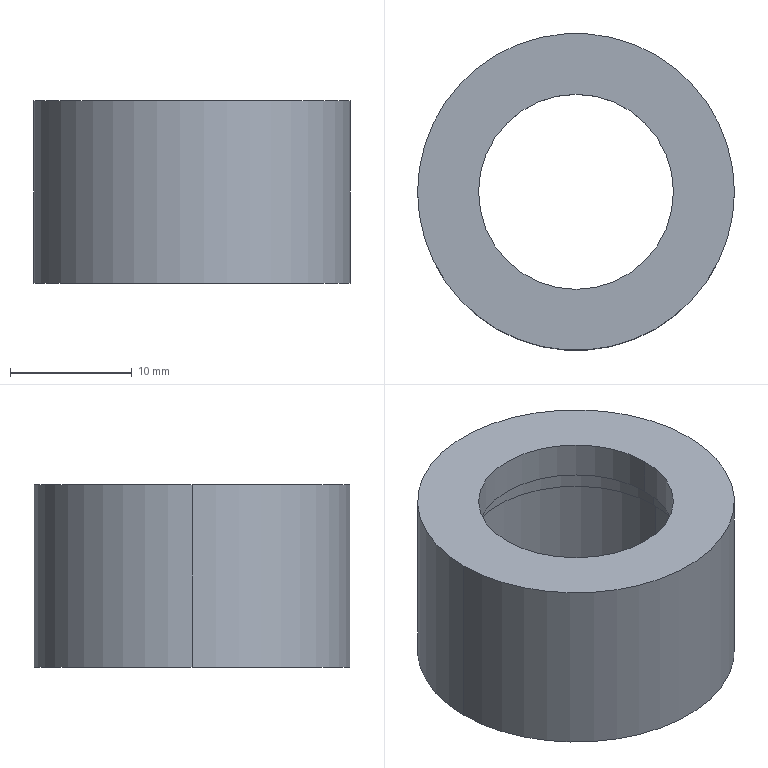Part | SolidWorks | features Revolution 1 | 1 solid | 13 faces | box 26 x 26 x 15 mm | volume 4163 mm3 | cylinder 8 | plane 3 | cone 2 | commonest cylinder face diameters 16 x2 18 x2 18.5 x2 26 x2
STEP:
#1=CARTESIAN_POINT('',(9.,0.,10.15));
#2=VERTEX_POINT('',#1);
#3=CARTESIAN_POINT('',(-9.,0.,10.15));
#4=VERTEX_POINT('',#3);
#5=CARTESIAN_POINT('',(0.,0.,10.15));
#6=DIRECTION('',(0.,0.,-1.));
#7=DIRECTION('',(-1.,0.,0.));
#8=AXIS2_PLACEMENT_3D('',#5,#6,#7);
#9=CIRCLE('',#8,9.);
#10=EDGE_CURVE('',#2,#4,#9,.T.);
#11=ORIENTED_EDGE('',*,*,#10,.F.);
#12=CARTESIAN_POINT('',(9.25,0.,10.));
#13=VERTEX_POINT('',#12);
#14=CARTESIAN_POINT('',(9.,0.,10.15));
#15=DIRECTION('',(0.8572,0.,-0.515));
#16=VECTOR('',#15,1000.);
#17=LINE('',#14,#16);
#18=EDGE_CURVE('',#2,#13,#17,.T.);
#19=ORIENTED_EDGE('',*,*,#18,.T.);
#20=CARTESIAN_POINT('',(-9.25,0.,10.));
#21=VERTEX_POINT('',#20);
#22=CARTESIAN_POINT('',(0.,0.,10.));
#23=DIRECTION('',(0.,0.,-1.));
#24=DIRECTION('',(-1.,0.,0.));
#25=AXIS2_PLACEMENT_3D('',#22,#23,#24);
#26=CIRCLE('',#25,9.25);
#27=EDGE_CURVE('',#13,#21,#26,.T.);
#28=ORIENTED_EDGE('',*,*,#27,.T.);
#29=CARTESIAN_POINT('',(-9.,0.,10.15));
#30=DIRECTION('',(-0.8572,0.,-0.515));
#31=VECTOR('',#30,1000.);
#32=LINE('',#29,#31);
#33=EDGE_CURVE('',#4,#21,#32,.T.);
#34=ORIENTED_EDGE('',*,*,#33,.F.);
#35=EDGE_LOOP('',(#11,#19,#28,#34));
#36=FACE_OUTER_BOUND('',#35,.T.);
#37=CARTESIAN_POINT('',(0.,0.,10.15));
#38=DIRECTION('',(0.,0.,-1.));
#39=DIRECTION('',(-1.,0.,0.));
#40=AXIS2_PLACEMENT_3D('',#37,#38,#39);
#41=CONICAL_SURFACE('',#40,9.,1.03);
#42=ADVANCED_FACE('',(#36),#41,.F.);
#43=CARTESIAN_POINT('',(9.,0.,12.));
#44=VERTEX_POINT('',#43);
#45=CARTESIAN_POINT('',(-9.,0.,12.));
#46=VERTEX_POINT('',#45);
#47=CARTESIAN_POINT('',(0.,0.,12.));
#48=DIRECTION('',(0.,0.,-1.));
#49=DIRECTION('',(-1.,0.,0.));
#50=AXIS2_PLACEMENT_3D('',#47,#48,#49);
#51=CIRCLE('',#50,9.);
#52=EDGE_CURVE('',#44,#46,#51,.T.);
#53=ORIENTED_EDGE('',*,*,#52,.F.);
#54=CARTESIAN_POINT('',(9.,0.,15.));
#55=DIRECTION('',(0.,0.,-1.));
#56=VECTOR('',#55,1000.);
#57=LINE('',#54,#56);
#58=EDGE_CURVE('',#44,#2,#57,.T.);
#59=ORIENTED_EDGE('',*,*,#58,.T.);
#60=ORIENTED_EDGE('',*,*,#10,.T.);
#61=CARTESIAN_POINT('',(-9.,0.,15.));
#62=DIRECTION('',(0.,0.,-1.));
#63=VECTOR('',#62,1000.);
#64=LINE('',#61,#63);
#65=EDGE_CURVE('',#46,#4,#64,.T.);
#66=ORIENTED_EDGE('',*,*,#65,.F.);
#67=EDGE_LOOP('',(#53,#59,#60,#66));
#68=FACE_OUTER_BOUND('',#67,.T.);
#69=CARTESIAN_POINT('',(0.,0.,15.));
#70=DIRECTION('',(0.,0.,-1.));
#71=DIRECTION('',(-1.,0.,0.));
#72=AXIS2_PLACEMENT_3D('',#69,#70,#71);
#73=CYLINDRICAL_SURFACE('',#72,9.);
#74=ADVANCED_FACE('',(#68),#73,.F.);
#75=CARTESIAN_POINT('',(8.,0.,15.));
#76=VERTEX_POINT('',#75);
#77=CARTESIAN_POINT('',(-8.,0.,15.));
#78=VERTEX_POINT('',#77);
#79=CARTESIAN_POINT('',(0.,0.,15.));
#80=DIRECTION('',(0.,0.,-1.));
#81=DIRECTION('',(-1.,0.,0.));
#82=AXIS2_PLACEMENT_3D('',#79,#80,#81);
#83=CIRCLE('',#82,8.);
#84=EDGE_CURVE('',#76,#78,#83,.T.);
#85=ORIENTED_EDGE('',*,*,#84,.F.);
#86=CARTESIAN_POINT('',(8.,0.,12.));
#87=VERTEX_POINT('',#86);
#88=CARTESIAN_POINT('',(8.,0.,15.));
#89=DIRECTION('',(0.,0.,-1.));
#90=VECTOR('',#89,1000.);
#91=LINE('',#88,#90);
#92=EDGE_CURVE('',#76,#87,#91,.T.);
#93=ORIENTED_EDGE('',*,*,#92,.T.);
#94=CARTESIAN_POINT('',(-8.,0.,12.));
#95=VERTEX_POINT('',#94);
#96=CARTESIAN_POINT('',(0.,0.,12.));
#97=DIRECTION('',(0.,0.,-1.));
#98=DIRECTION('',(-1.,0.,0.));
#99=AXIS2_PLACEMENT_3D('',#96,#97,#98);
#100=CIRCLE('',#99,8.);
#101=EDGE_CURVE('',#87,#95,#100,.T.);
#102=ORIENTED_EDGE('',*,*,#101,.T.);
#103=CARTESIAN_POINT('',(-8.,0.,15.));
#104=DIRECTION('',(0.,0.,-1.));
#105=VECTOR('',#104,1000.);
#106=LINE('',#103,#105);
#107=EDGE_CURVE('',#78,#95,#106,.T.);
#108=ORIENTED_EDGE('',*,*,#107,.F.);
#109=EDGE_LOOP('',(#85,#93,#102,#108));
#110=FACE_OUTER_BOUND('',#109,.T.);
#111=CARTESIAN_POINT('',(0.,0.,15.));
#112=DIRECTION('',(0.,0.,-1.));
#113=DIRECTION('',(-1.,0.,0.));
#114=AXIS2_PLACEMENT_3D('',#111,#112,#113);
#115=CYLINDRICAL_SURFACE('',#114,8.);
#116=ADVANCED_FACE('',(#110),#115,.F.);
#117=CARTESIAN_POINT('',(-13.,0.,15.));
#118=VERTEX_POINT('',#117);
#119=CARTESIAN_POINT('',(13.,0.,15.));
#120=VERTEX_POINT('',#119);
#121=CARTESIAN_POINT('',(0.,0.,15.));
#122=DIRECTION('',(0.,0.,-1.));
#123=DIRECTION('',(-1.,0.,0.));
#124=AXIS2_PLACEMENT_3D('',#121,#122,#123);
#125=CIRCLE('',#124,13.);
#126=EDGE_CURVE('',#118,#120,#125,.T.);
#127=ORIENTED_EDGE('',*,*,#126,.T.);
#128=CARTESIAN_POINT('',(13.,0.,0.));
#129=VERTEX_POINT('',#128);
#130=CARTESIAN_POINT('',(13.,0.,15.));
#131=DIRECTION('',(0.,0.,-1.));
#132=VECTOR('',#131,1000.);
#133=LINE('',#130,#132);
#134=EDGE_CURVE('',#120,#129,#133,.T.);
#135=ORIENTED_EDGE('',*,*,#134,.T.);
#136=CARTESIAN_POINT('',(-13.,0.,0.));
#137=VERTEX_POINT('',#136);
#138=CARTESIAN_POINT('',(0.,0.,0.));
#139=DIRECTION('',(0.,0.,-1.));
#140=DIRECTION('',(-1.,0.,0.));
#141=AXIS2_PLACEMENT_3D('',#138,#139,#140);
#142=CIRCLE('',#141,13.);
#143=EDGE_CURVE('',#137,#129,#142,.T.);
#144=ORIENTED_EDGE('',*,*,#143,.F.);
#145=CARTESIAN_POINT('',(-13.,0.,15.));
#146=DIRECTION('',(0.,0.,-1.));
#147=VECTOR('',#146,1000.);
#148=LINE('',#145,#147);
#149=EDGE_CURVE('',#118,#137,#148,.T.);
#150=ORIENTED_EDGE('',*,*,#149,.F.);
#151=EDGE_LOOP('',(#127,#135,#144,#150));
#152=FACE_OUTER_BOUND('',#151,.T.);
#153=CARTESIAN_POINT('',(0.,0.,15.));
#154=DIRECTION('',(0.,0.,-1.));
#155=DIRECTION('',(-1.,0.,0.));
#156=AXIS2_PLACEMENT_3D('',#153,#154,#155);
#157=CYLINDRICAL_SURFACE('',#156,13.);
#158=ADVANCED_FACE('',(#152),#157,.T.);
#159=ORIENTED_EDGE('',*,*,#27,.F.);
#160=CARTESIAN_POINT('',(9.25,0.,0.));
#161=VERTEX_POINT('',#160);
#162=CARTESIAN_POINT('',(9.25,0.,15.));
#163=DIRECTION('',(0.,0.,-1.));
#164=VECTOR('',#163,1000.);
#165=LINE('',#162,#164);
#166=EDGE_CURVE('',#13,#161,#165,.T.);
#167=ORIENTED_EDGE('',*,*,#166,.T.);
#168=CARTESIAN_POINT('',(-9.25,0.,0.));
#169=VERTEX_POINT('',#168);
#170=CARTESIAN_POINT('',(0.,0.,0.));
#171=DIRECTION('',(0.,0.,-1.));
#172=DIRECTION('',(-1.,0.,0.));
#173=AXIS2_PLACEMENT_3D('',#170,#171,#172);
#174=CIRCLE('',#173,9.25);
#175=EDGE_CURVE('',#161,#169,#174,.T.);
#176=ORIENTED_EDGE('',*,*,#175,.T.);
#177=CARTESIAN_POINT('',(-9.25,0.,15.));
#178=DIRECTION('',(0.,0.,-1.));
#179=VECTOR('',#178,1000.);
#180=LINE('',#177,#179);
#181=EDGE_CURVE('',#21,#169,#180,.T.);
#182=ORIENTED_EDGE('',*,*,#181,.F.);
#183=EDGE_LOOP('',(#159,#167,#176,#182));
#184=FACE_OUTER_BOUND('',#183,.T.);
#185=CARTESIAN_POINT('',(0.,0.,15.));
#186=DIRECTION('',(0.,0.,-1.));
#187=DIRECTION('',(-1.,0.,0.));
#188=AXIS2_PLACEMENT_3D('',#185,#186,#187);
#189=CYLINDRICAL_SURFACE('',#188,9.25);
#190=ADVANCED_FACE('',(#184),#189,.F.);
#191=ORIENTED_EDGE('',*,*,#166,.F.);
#192=CARTESIAN_POINT('',(0.,0.,10.));
#193=DIRECTION('',(0.,0.,-1.));
#194=DIRECTION('',(-1.,0.,0.));
#195=AXIS2_PLACEMENT_3D('',#192,#193,#194);
#196=CIRCLE('',#195,9.25);
#197=EDGE_CURVE('',#21,#13,#196,.T.);
#198=ORIENTED_EDGE('',*,*,#197,.F.);
#199=ORIENTED_EDGE('',*,*,#181,.T.);
#200=CARTESIAN_POINT('',(0.,0.,0.));
#201=DIRECTION('',(0.,0.,-1.));
#202=DIRECTION('',(-1.,0.,0.));
#203=AXIS2_PLACEMENT_3D('',#200,#201,#202);
#204=CIRCLE('',#203,9.25);
#205=EDGE_CURVE('',#169,#161,#204,.T.);
#206=ORIENTED_EDGE('',*,*,#205,.T.);
#207=EDGE_LOOP('',(#191,#198,#199,#206));
#208=FACE_OUTER_BOUND('',#207,.T.);
#209=CARTESIAN_POINT('',(0.,0.,15.));
#210=DIRECTION('',(0.,0.,-1.));
#211=DIRECTION('',(-1.,0.,0.));
#212=AXIS2_PLACEMENT_3D('',#209,#210,#211);
#213=CYLINDRICAL_SURFACE('',#212,9.25);
#214=ADVANCED_FACE('',(#208),#213,.F.);
#215=ORIENTED_EDGE('',*,*,#143,.T.);
#216=CARTESIAN_POINT('',(0.,0.,0.));
#217=DIRECTION('',(0.,0.,-1.));
#218=DIRECTION('',(-1.,0.,0.));
#219=AXIS2_PLACEMENT_3D('',#216,#217,#218);
#220=CIRCLE('',#219,13.);
#221=EDGE_CURVE('',#129,#137,#220,.T.);
#222=ORIENTED_EDGE('',*,*,#221,.T.);
#223=EDGE_LOOP('',(#215,#222));
#224=FACE_OUTER_BOUND('',#223,.T.);
#225=ORIENTED_EDGE('',*,*,#205,.F.);
#226=ORIENTED_EDGE('',*,*,#175,.F.);
#227=EDGE_LOOP('',(#225,#226));
#228=FACE_BOUND('',#227,.T.);
#229=CARTESIAN_POINT('',(9.25,0.,0.));
#230=DIRECTION('',(0.,0.,-1.));
#231=DIRECTION('',(-1.,0.,0.));
#232=AXIS2_PLACEMENT_3D('',#229,#230,#231);
#233=PLANE('',#232);
#234=ADVANCED_FACE('',(#224,#228),#233,.T.);
#235=ORIENTED_EDGE('',*,*,#134,.F.);
#236=CARTESIAN_POINT('',(0.,0.,15.));
#237=DIRECTION('',(0.,0.,-1.));
#238=DIRECTION('',(-1.,0.,0.));
#239=AXIS2_PLACEMENT_3D('',#236,#237,#238);
#240=CIRCLE('',#239,13.);
#241=EDGE_CURVE('',#120,#118,#240,.T.);
#242=ORIENTED_EDGE('',*,*,#241,.T.);
#243=ORIENTED_EDGE('',*,*,#149,.T.);
#244=ORIENTED_EDGE('',*,*,#221,.F.);
#245=EDGE_LOOP('',(#235,#242,#243,#244));
#246=FACE_OUTER_BOUND('',#245,.T.);
#247=CARTESIAN_POINT('',(0.,0.,15.));
#248=DIRECTION('',(0.,0.,-1.));
#249=DIRECTION('',(-1.,0.,0.));
#250=AXIS2_PLACEMENT_3D('',#247,#248,#249);
#251=CYLINDRICAL_SURFACE('',#250,13.);
#252=ADVANCED_FACE('',(#246),#251,.T.);
#253=CARTESIAN_POINT('',(0.,0.,15.));
#254=DIRECTION('',(0.,0.,-1.));
#255=DIRECTION('',(-1.,0.,0.));
#256=AXIS2_PLACEMENT_3D('',#253,#254,#255);
#257=CIRCLE('',#256,8.);
#258=EDGE_CURVE('',#78,#76,#257,.T.);
#259=ORIENTED_EDGE('',*,*,#258,.T.);
#260=ORIENTED_EDGE('',*,*,#84,.T.);
#261=EDGE_LOOP('',(#259,#260));
#262=FACE_BOUND('',#261,.T.);
#263=ORIENTED_EDGE('',*,*,#126,.F.);
#264=ORIENTED_EDGE('',*,*,#241,.F.);
#265=EDGE_LOOP('',(#263,#264));
#266=FACE_OUTER_BOUND('',#265,.T.);
#267=CARTESIAN_POINT('',(13.,0.,15.));
#268=DIRECTION('',(0.,0.,1.));
#269=DIRECTION('',(1.,0.,0.));
#270=AXIS2_PLACEMENT_3D('',#267,#268,#269);
#271=PLANE('',#270);
#272=ADVANCED_FACE('',(#262,#266),#271,.T.);
#273=ORIENTED_EDGE('',*,*,#92,.F.);
#274=ORIENTED_EDGE('',*,*,#258,.F.);
#275=ORIENTED_EDGE('',*,*,#107,.T.);
#276=CARTESIAN_POINT('',(0.,0.,12.));
#277=DIRECTION('',(0.,0.,-1.));
#278=DIRECTION('',(-1.,0.,0.));
#279=AXIS2_PLACEMENT_3D('',#276,#277,#278);
#280=CIRCLE('',#279,8.);
#281=EDGE_CURVE('',#95,#87,#280,.T.);
#282=ORIENTED_EDGE('',*,*,#281,.T.);
#283=EDGE_LOOP('',(#273,#274,#275,#282));
#284=FACE_OUTER_BOUND('',#283,.T.);
#285=CARTESIAN_POINT('',(0.,0.,15.));
#286=DIRECTION('',(0.,0.,-1.));
#287=DIRECTION('',(-1.,0.,0.));
#288=AXIS2_PLACEMENT_3D('',#285,#286,#287);
#289=CYLINDRICAL_SURFACE('',#288,8.);
#290=ADVANCED_FACE('',(#284),#289,.F.);
#291=CARTESIAN_POINT('',(0.,0.,12.));
#292=DIRECTION('',(0.,0.,-1.));
#293=DIRECTION('',(-1.,0.,0.));
#294=AXIS2_PLACEMENT_3D('',#291,#292,#293);
#295=CIRCLE('',#294,9.);
#296=EDGE_CURVE('',#46,#44,#295,.T.);
#297=ORIENTED_EDGE('',*,*,#296,.T.);
#298=ORIENTED_EDGE('',*,*,#52,.T.);
#299=EDGE_LOOP('',(#297,#298));
#300=FACE_OUTER_BOUND('',#299,.T.);
#301=ORIENTED_EDGE('',*,*,#281,.F.);
#302=ORIENTED_EDGE('',*,*,#101,.F.);
#303=EDGE_LOOP('',(#301,#302));
#304=FACE_BOUND('',#303,.T.);
#305=CARTESIAN_POINT('',(8.,0.,12.));
#306=DIRECTION('',(0.,0.,-1.));
#307=DIRECTION('',(-1.,0.,0.));
#308=AXIS2_PLACEMENT_3D('',#305,#306,#307);
#309=PLANE('',#308);
#310=ADVANCED_FACE('',(#300,#304),#309,.T.);
#311=ORIENTED_EDGE('',*,*,#58,.F.);
#312=ORIENTED_EDGE('',*,*,#296,.F.);
#313=ORIENTED_EDGE('',*,*,#65,.T.);
#314=CARTESIAN_POINT('',(0.,0.,10.15));
#315=DIRECTION('',(0.,0.,-1.));
#316=DIRECTION('',(-1.,0.,0.));
#317=AXIS2_PLACEMENT_3D('',#314,#315,#316);
#318=CIRCLE('',#317,9.);
#319=EDGE_CURVE('',#4,#2,#318,.T.);
#320=ORIENTED_EDGE('',*,*,#319,.T.);
#321=EDGE_LOOP('',(#311,#312,#313,#320));
#322=FACE_OUTER_BOUND('',#321,.T.);
#323=CARTESIAN_POINT('',(0.,0.,15.));
#324=DIRECTION('',(0.,0.,-1.));
#325=DIRECTION('',(-1.,0.,0.));
#326=AXIS2_PLACEMENT_3D('',#323,#324,#325);
#327=CYLINDRICAL_SURFACE('',#326,9.);
#328=ADVANCED_FACE('',(#322),#327,.F.);
#329=ORIENTED_EDGE('',*,*,#18,.F.);
#330=ORIENTED_EDGE('',*,*,#319,.F.);
#331=ORIENTED_EDGE('',*,*,#33,.T.);
#332=ORIENTED_EDGE('',*,*,#197,.T.);
#333=EDGE_LOOP('',(#329,#330,#331,#332));
#334=FACE_OUTER_BOUND('',#333,.T.);
#335=CARTESIAN_POINT('',(0.,0.,10.15));
#336=DIRECTION('',(0.,0.,-1.));
#337=DIRECTION('',(-1.,0.,0.));
#338=AXIS2_PLACEMENT_3D('',#335,#336,#337);
#339=CONICAL_SURFACE('',#338,9.,1.03);
#340=ADVANCED_FACE('',(#334),#339,.F.);
#341=CLOSED_SHELL('',(#42,#74,#116,#158,#190,#214,#234,#252,#272,#290,#310,#328,#340));
#342=MANIFOLD_SOLID_BREP('',#341);
#343=CARTESIAN_POINT('',(0.,0.,0.));
#344=DIRECTION('',(0.,0.,1.));
#345=DIRECTION('',(1.,0.,0.));
#346=AXIS2_PLACEMENT_3D('',#343,#344,#345);
#347=(LENGTH_UNIT()NAMED_UNIT(*)SI_UNIT(.MILLI.,.METRE.));
#348=UNCERTAINTY_MEASURE_WITH_UNIT(LENGTH_MEASURE(0.00001),#347,'','');
#349=(NAMED_UNIT(*)PLANE_ANGLE_UNIT()SI_UNIT($,.RADIAN.));
#350=(NAMED_UNIT(*)SI_UNIT($,.STERADIAN.)SOLID_ANGLE_UNIT());
#351=(GEOMETRIC_REPRESENTATION_CONTEXT(3)GLOBAL_UNCERTAINTY_ASSIGNED_CONTEXT((#348))GLOBAL_UNIT_ASSIGNED_CONTEXT((#347,#349,#350))REPRESENTATION_CONTEXT('',''));
#352=ADVANCED_BREP_SHAPE_REPRESENTATION('',(#342,#346),#351);